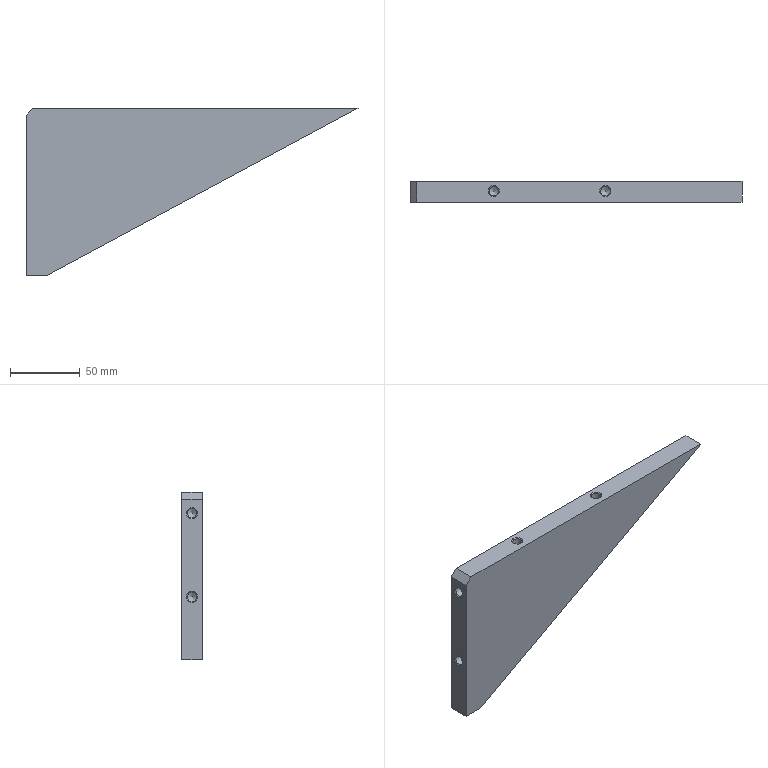Part | STEP file | YBQDJ-FLJ-6 | 1 solid | 19 faces | box 237.857 x 15 x 120 mm | volume 224363 mm3 | cone 8 | plane 7 | cylinder 4 | commonest cylinder face diameters 6.8 x4
STEP:
#1=CARTESIAN_POINT('',(0.,0.,0.));
#2=DIRECTION('',(0.,0.,1.));
#3=DIRECTION('',(1.,0.,0.));
#4=AXIS2_PLACEMENT_3D('',#1,#2,#3);
#5=CARTESIAN_POINT('',(486.5,-270.,-240.));
#6=VERTEX_POINT('',#5);
#7=CARTESIAN_POINT('',(486.5,-270.,-355.));
#8=VERTEX_POINT('',#7);
#9=CARTESIAN_POINT('',(486.5,-270.,-235.));
#10=DIRECTION('',(0.,0.,-1.));
#11=VECTOR('',#10,1.);
#12=LINE('',#9,#11);
#13=CARTESIAN_POINT('',(666.5,-270.,-395.));
#14=DIRECTION('',(0.,-1.,0.));
#15=DIRECTION('',(0.,0.,-1.));
#16=AXIS2_PLACEMENT_3D('',#13,#14,#15);
#17=PLANE('',#16);
#18=CARTESIAN_POINT('',(-160.,-180.));
#19=DIRECTION('',(1.,0.));
#20=VECTOR('',#19,1.);
#21=LINE('',#18,#20);
#22=(GEOMETRIC_REPRESENTATION_CONTEXT(2)PARAMETRIC_REPRESENTATION_CONTEXT()REPRESENTATION_CONTEXT('',''));
#23=DEFINITIONAL_REPRESENTATION('',(#21),#22);
#24=PCURVE('',#17,#23);
#25=CARTESIAN_POINT('',(486.5,-136.5,-235.));
#26=DIRECTION('',(-1.,0.,0.));
#27=DIRECTION('',(0.,0.,1.));
#28=AXIS2_PLACEMENT_3D('',#25,#26,#27);
#29=PLANE('',#28);
#30=CARTESIAN_POINT('',(0.,-133.5));
#31=DIRECTION('',(-1.,0.));
#32=VECTOR('',#31,1.);
#33=LINE('',#30,#32);
#34=(GEOMETRIC_REPRESENTATION_CONTEXT(2)PARAMETRIC_REPRESENTATION_CONTEXT()REPRESENTATION_CONTEXT('',''));
#35=DEFINITIONAL_REPRESENTATION('',(#33),#34);
#36=PCURVE('',#29,#35);
#37=SURFACE_CURVE('',#12,(#24,#36),.PCURVE_S1.);
#38=EDGE_CURVE('',#6,#8,#37,.T.);
#39=ORIENTED_EDGE('',*,*,#38,.F.);
#40=CARTESIAN_POINT('',(491.5,-270.,-235.));
#41=VERTEX_POINT('',#40);
#42=CARTESIAN_POINT('',(499.,-270.,-227.5));
#43=DIRECTION('',(0.7071,0.,0.7071));
#44=VECTOR('',#43,1.);
#45=LINE('',#42,#44);
#46=CARTESIAN_POINT('',(-167.5,-167.5));
#47=DIRECTION('',(-0.7071,0.7071));
#48=VECTOR('',#47,1.);
#49=LINE('',#46,#48);
#50=(GEOMETRIC_REPRESENTATION_CONTEXT(2)PARAMETRIC_REPRESENTATION_CONTEXT()REPRESENTATION_CONTEXT('',''));
#51=DEFINITIONAL_REPRESENTATION('',(#49),#50);
#52=PCURVE('',#17,#51);
#53=CARTESIAN_POINT('',(491.5,-136.5,-235.));
#54=DIRECTION('',(0.7071,0.,-0.7071));
#55=DIRECTION('',(0.,-1.,0.));
#56=AXIS2_PLACEMENT_3D('',#53,#54,#55);
#57=PLANE('',#56);
#58=CARTESIAN_POINT('',(133.5,-10.607));
#59=DIRECTION('',(0.,-1.));
#60=VECTOR('',#59,1.);
#61=LINE('',#58,#60);
#62=(GEOMETRIC_REPRESENTATION_CONTEXT(2)PARAMETRIC_REPRESENTATION_CONTEXT()REPRESENTATION_CONTEXT('',''));
#63=DEFINITIONAL_REPRESENTATION('',(#61),#62);
#64=PCURVE('',#57,#63);
#65=SURFACE_CURVE('',#45,(#52,#64),.PCURVE_S1.);
#66=EDGE_CURVE('',#6,#41,#65,.T.);
#67=ORIENTED_EDGE('',*,*,#66,.T.);
#68=CARTESIAN_POINT('',(724.357,-270.,-235.));
#69=VERTEX_POINT('',#68);
#70=CARTESIAN_POINT('',(696.5,-270.,-235.));
#71=DIRECTION('',(-1.,0.,0.));
#72=VECTOR('',#71,1.);
#73=LINE('',#70,#72);
#74=CARTESIAN_POINT('',(-160.,30.));
#75=DIRECTION('',(0.,-1.));
#76=VECTOR('',#75,1.);
#77=LINE('',#74,#76);
#78=(GEOMETRIC_REPRESENTATION_CONTEXT(2)PARAMETRIC_REPRESENTATION_CONTEXT()REPRESENTATION_CONTEXT('',''));
#79=DEFINITIONAL_REPRESENTATION('',(#77),#78);
#80=PCURVE('',#17,#79);
#81=CARTESIAN_POINT('',(696.5,-136.5,-235.));
#82=DIRECTION('',(0.,0.,1.));
#83=DIRECTION('',(1.,0.,0.));
#84=AXIS2_PLACEMENT_3D('',#81,#82,#83);
#85=PLANE('',#84);
#86=CARTESIAN_POINT('',(0.,-133.5));
#87=DIRECTION('',(-1.,0.));
#88=VECTOR('',#87,1.);
#89=LINE('',#86,#88);
#90=(GEOMETRIC_REPRESENTATION_CONTEXT(2)PARAMETRIC_REPRESENTATION_CONTEXT()REPRESENTATION_CONTEXT('',''));
#91=DEFINITIONAL_REPRESENTATION('',(#89),#90);
#92=PCURVE('',#85,#91);
#93=SURFACE_CURVE('',#73,(#80,#92),.PCURVE_S1.);
#94=EDGE_CURVE('',#69,#41,#93,.T.);
#95=ORIENTED_EDGE('',*,*,#94,.F.);
#96=CARTESIAN_POINT('',(501.5,-270.,-355.));
#97=VERTEX_POINT('',#96);
#98=CARTESIAN_POINT('',(501.5,-270.,-355.));
#99=DIRECTION('',(0.8805,0.,0.4741));
#100=VECTOR('',#99,1.);
#101=LINE('',#98,#100);
#102=CARTESIAN_POINT('',(-40.,-165.));
#103=DIRECTION('',(-0.4741,0.8805));
#104=VECTOR('',#103,1.);
#105=LINE('',#102,#104);
#106=(GEOMETRIC_REPRESENTATION_CONTEXT(2)PARAMETRIC_REPRESENTATION_CONTEXT()REPRESENTATION_CONTEXT('',''));
#107=DEFINITIONAL_REPRESENTATION('',(#105),#106);
#108=PCURVE('',#17,#107);
#109=CARTESIAN_POINT('',(501.5,-136.5,-355.));
#110=DIRECTION('',(0.4741,0.,-0.8805));
#111=DIRECTION('',(-0.8805,0.,-0.4741));
#112=AXIS2_PLACEMENT_3D('',#109,#110,#111);
#113=PLANE('',#112);
#114=CARTESIAN_POINT('',(0.,-133.5));
#115=DIRECTION('',(-1.,0.));
#116=VECTOR('',#115,1.);
#117=LINE('',#114,#116);
#118=(GEOMETRIC_REPRESENTATION_CONTEXT(2)PARAMETRIC_REPRESENTATION_CONTEXT()REPRESENTATION_CONTEXT('',''));
#119=DEFINITIONAL_REPRESENTATION('',(#117),#118);
#120=PCURVE('',#113,#119);
#121=SURFACE_CURVE('',#101,(#108,#120),.PCURVE_S1.);
#122=EDGE_CURVE('',#97,#69,#121,.T.);
#123=ORIENTED_EDGE('',*,*,#122,.F.);
#124=CARTESIAN_POINT('',(486.5,-270.,-355.));
#125=DIRECTION('',(1.,0.,0.));
#126=VECTOR('',#125,1.);
#127=LINE('',#124,#126);
#128=CARTESIAN_POINT('',(-40.,-180.));
#129=DIRECTION('',(0.,1.));
#130=VECTOR('',#129,1.);
#131=LINE('',#128,#130);
#132=(GEOMETRIC_REPRESENTATION_CONTEXT(2)PARAMETRIC_REPRESENTATION_CONTEXT()REPRESENTATION_CONTEXT('',''));
#133=DEFINITIONAL_REPRESENTATION('',(#131),#132);
#134=PCURVE('',#17,#133);
#135=CARTESIAN_POINT('',(486.5,-136.5,-355.));
#136=DIRECTION('',(0.,0.,-1.));
#137=DIRECTION('',(-1.,0.,0.));
#138=AXIS2_PLACEMENT_3D('',#135,#136,#137);
#139=PLANE('',#138);
#140=CARTESIAN_POINT('',(0.,-133.5));
#141=DIRECTION('',(-1.,0.));
#142=VECTOR('',#141,1.);
#143=LINE('',#140,#142);
#144=(GEOMETRIC_REPRESENTATION_CONTEXT(2)PARAMETRIC_REPRESENTATION_CONTEXT()REPRESENTATION_CONTEXT('',''));
#145=DEFINITIONAL_REPRESENTATION('',(#143),#144);
#146=PCURVE('',#139,#145);
#147=SURFACE_CURVE('',#127,(#134,#146),.PCURVE_S1.);
#148=EDGE_CURVE('',#8,#97,#147,.T.);
#149=ORIENTED_EDGE('',*,*,#148,.F.);
#150=EDGE_LOOP('',(#39,#67,#95,#123,#149));
#151=FACE_BOUND('',#150,.T.);
#152=ADVANCED_FACE('',(#151),#17,.F.);
#153=CARTESIAN_POINT('',(486.5,-285.,-355.));
#154=VERTEX_POINT('',#153);
#155=CARTESIAN_POINT('',(486.5,-136.5,-355.));
#156=DIRECTION('',(0.,-1.,0.));
#157=VECTOR('',#156,1.);
#158=LINE('',#155,#157);
#159=CARTESIAN_POINT('',(0.,0.));
#160=DIRECTION('',(0.,-1.));
#161=VECTOR('',#160,1.);
#162=LINE('',#159,#161);
#163=(GEOMETRIC_REPRESENTATION_CONTEXT(2)PARAMETRIC_REPRESENTATION_CONTEXT()REPRESENTATION_CONTEXT('',''));
#164=DEFINITIONAL_REPRESENTATION('',(#162),#163);
#165=PCURVE('',#139,#164);
#166=CARTESIAN_POINT('',(-120.,0.));
#167=DIRECTION('',(0.,-1.));
#168=VECTOR('',#167,1.);
#169=LINE('',#166,#168);
#170=(GEOMETRIC_REPRESENTATION_CONTEXT(2)PARAMETRIC_REPRESENTATION_CONTEXT()REPRESENTATION_CONTEXT('',''));
#171=DEFINITIONAL_REPRESENTATION('',(#169),#170);
#172=PCURVE('',#29,#171);
#173=SURFACE_CURVE('',#158,(#165,#172),.PCURVE_S1.);
#174=EDGE_CURVE('',#8,#154,#173,.T.);
#175=ORIENTED_EDGE('',*,*,#174,.F.);
#176=ORIENTED_EDGE('',*,*,#148,.T.);
#177=CARTESIAN_POINT('',(501.5,-285.,-355.));
#178=VERTEX_POINT('',#177);
#179=CARTESIAN_POINT('',(501.5,-136.5,-355.));
#180=DIRECTION('',(0.,-1.,0.));
#181=VECTOR('',#180,1.);
#182=LINE('',#179,#181);
#183=CARTESIAN_POINT('',(-15.,0.));
#184=DIRECTION('',(0.,-1.));
#185=VECTOR('',#184,1.);
#186=LINE('',#183,#185);
#187=(GEOMETRIC_REPRESENTATION_CONTEXT(2)PARAMETRIC_REPRESENTATION_CONTEXT()REPRESENTATION_CONTEXT('',''));
#188=DEFINITIONAL_REPRESENTATION('',(#186),#187);
#189=PCURVE('',#139,#188);
#190=CARTESIAN_POINT('',(0.,0.));
#191=DIRECTION('',(0.,-1.));
#192=VECTOR('',#191,1.);
#193=LINE('',#190,#192);
#194=(GEOMETRIC_REPRESENTATION_CONTEXT(2)PARAMETRIC_REPRESENTATION_CONTEXT()REPRESENTATION_CONTEXT('',''));
#195=DEFINITIONAL_REPRESENTATION('',(#193),#194);
#196=PCURVE('',#113,#195);
#197=SURFACE_CURVE('',#182,(#189,#196),.PCURVE_S1.);
#198=EDGE_CURVE('',#97,#178,#197,.T.);
#199=ORIENTED_EDGE('',*,*,#198,.T.);
#200=CARTESIAN_POINT('',(486.5,-285.,-355.));
#201=DIRECTION('',(1.,0.,0.));
#202=VECTOR('',#201,1.);
#203=LINE('',#200,#202);
#204=CARTESIAN_POINT('',(0.,-148.5));
#205=DIRECTION('',(-1.,0.));
#206=VECTOR('',#205,1.);
#207=LINE('',#204,#206);
#208=(GEOMETRIC_REPRESENTATION_CONTEXT(2)PARAMETRIC_REPRESENTATION_CONTEXT()REPRESENTATION_CONTEXT('',''));
#209=DEFINITIONAL_REPRESENTATION('',(#207),#208);
#210=PCURVE('',#139,#209);
#211=CARTESIAN_POINT('',(-13.5,-285.,-95.));
#212=DIRECTION('',(0.,1.,0.));
#213=DIRECTION('',(0.,0.,1.));
#214=AXIS2_PLACEMENT_3D('',#211,#212,#213);
#215=PLANE('',#214);
#216=CARTESIAN_POINT('',(-260.,500.));
#217=DIRECTION('',(0.,1.));
#218=VECTOR('',#217,1.);
#219=LINE('',#216,#218);
#220=(GEOMETRIC_REPRESENTATION_CONTEXT(2)PARAMETRIC_REPRESENTATION_CONTEXT()REPRESENTATION_CONTEXT('',''));
#221=DEFINITIONAL_REPRESENTATION('',(#219),#220);
#222=PCURVE('',#215,#221);
#223=SURFACE_CURVE('',#203,(#210,#222),.PCURVE_S1.);
#224=EDGE_CURVE('',#154,#178,#223,.T.);
#225=ORIENTED_EDGE('',*,*,#224,.F.);
#226=EDGE_LOOP('',(#175,#176,#199,#225));
#227=FACE_BOUND('',#226,.T.);
#228=ADVANCED_FACE('',(#227),#139,.T.);
#229=ORIENTED_EDGE('',*,*,#198,.F.);
#230=ORIENTED_EDGE('',*,*,#122,.T.);
#231=CARTESIAN_POINT('',(724.357,-285.,-235.));
#232=VERTEX_POINT('',#231);
#233=CARTESIAN_POINT('',(724.357,-136.5,-235.));
#234=DIRECTION('',(0.,1.,0.));
#235=VECTOR('',#234,1.);
#236=LINE('',#233,#235);
#237=CARTESIAN_POINT('',(-253.111,0.));
#238=DIRECTION('',(0.,1.));
#239=VECTOR('',#238,1.);
#240=LINE('',#237,#239);
#241=(GEOMETRIC_REPRESENTATION_CONTEXT(2)PARAMETRIC_REPRESENTATION_CONTEXT()REPRESENTATION_CONTEXT('',''));
#242=DEFINITIONAL_REPRESENTATION('',(#240),#241);
#243=PCURVE('',#113,#242);
#244=CARTESIAN_POINT('',(27.857,0.));
#245=DIRECTION('',(0.,1.));
#246=VECTOR('',#245,1.);
#247=LINE('',#244,#246);
#248=(GEOMETRIC_REPRESENTATION_CONTEXT(2)PARAMETRIC_REPRESENTATION_CONTEXT()REPRESENTATION_CONTEXT('',''));
#249=DEFINITIONAL_REPRESENTATION('',(#247),#248);
#250=PCURVE('',#85,#249);
#251=SURFACE_CURVE('',#236,(#243,#250),.PCURVE_S1.);
#252=EDGE_CURVE('',#232,#69,#251,.T.);
#253=ORIENTED_EDGE('',*,*,#252,.F.);
#254=CARTESIAN_POINT('',(501.5,-285.,-355.));
#255=DIRECTION('',(0.8805,0.,0.4741));
#256=VECTOR('',#255,1.);
#257=LINE('',#254,#256);
#258=CARTESIAN_POINT('',(0.,-148.5));
#259=DIRECTION('',(-1.,0.));
#260=VECTOR('',#259,1.);
#261=LINE('',#258,#260);
#262=(GEOMETRIC_REPRESENTATION_CONTEXT(2)PARAMETRIC_REPRESENTATION_CONTEXT()REPRESENTATION_CONTEXT('',''));
#263=DEFINITIONAL_REPRESENTATION('',(#261),#262);
#264=PCURVE('',#113,#263);
#265=CARTESIAN_POINT('',(-260.,515.));
#266=DIRECTION('',(0.4741,0.8805));
#267=VECTOR('',#266,1.);
#268=LINE('',#265,#267);
#269=(GEOMETRIC_REPRESENTATION_CONTEXT(2)PARAMETRIC_REPRESENTATION_CONTEXT()REPRESENTATION_CONTEXT('',''));
#270=DEFINITIONAL_REPRESENTATION('',(#268),#269);
#271=PCURVE('',#215,#270);
#272=SURFACE_CURVE('',#257,(#264,#271),.PCURVE_S1.);
#273=EDGE_CURVE('',#178,#232,#272,.T.);
#274=ORIENTED_EDGE('',*,*,#273,.F.);
#275=EDGE_LOOP('',(#229,#230,#253,#274));
#276=FACE_BOUND('',#275,.T.);
#277=ADVANCED_FACE('',(#276),#113,.T.);
#278=CARTESIAN_POINT('',(491.5,-285.,-235.));
#279=VERTEX_POINT('',#278);
#280=CARTESIAN_POINT('',(696.5,-285.,-235.));
#281=DIRECTION('',(-1.,0.,0.));
#282=VECTOR('',#281,1.);
#283=LINE('',#280,#282);
#284=CARTESIAN_POINT('',(-140.,710.));
#285=DIRECTION('',(0.,-1.));
#286=VECTOR('',#285,1.);
#287=LINE('',#284,#286);
#288=(GEOMETRIC_REPRESENTATION_CONTEXT(2)PARAMETRIC_REPRESENTATION_CONTEXT()REPRESENTATION_CONTEXT('',''));
#289=DEFINITIONAL_REPRESENTATION('',(#287),#288);
#290=PCURVE('',#215,#289);
#291=CARTESIAN_POINT('',(0.,-148.5));
#292=DIRECTION('',(-1.,0.));
#293=VECTOR('',#292,1.);
#294=LINE('',#291,#293);
#295=(GEOMETRIC_REPRESENTATION_CONTEXT(2)PARAMETRIC_REPRESENTATION_CONTEXT()REPRESENTATION_CONTEXT('',''));
#296=DEFINITIONAL_REPRESENTATION('',(#294),#295);
#297=PCURVE('',#85,#296);
#298=SURFACE_CURVE('',#283,(#290,#297),.PCURVE_S1.);
#299=EDGE_CURVE('',#232,#279,#298,.T.);
#300=ORIENTED_EDGE('',*,*,#299,.T.);
#301=CARTESIAN_POINT('',(486.5,-285.,-240.));
#302=VERTEX_POINT('',#301);
#303=CARTESIAN_POINT('',(491.5,-285.,-235.));
#304=DIRECTION('',(-0.7071,0.,-0.7071));
#305=VECTOR('',#304,1.);
#306=LINE('',#303,#305);
#307=CARTESIAN_POINT('',(-140.,505.));
#308=DIRECTION('',(-0.7071,-0.7071));
#309=VECTOR('',#308,1.);
#310=LINE('',#307,#309);
#311=(GEOMETRIC_REPRESENTATION_CONTEXT(2)PARAMETRIC_REPRESENTATION_CONTEXT()REPRESENTATION_CONTEXT('',''));
#312=DEFINITIONAL_REPRESENTATION('',(#310),#311);
#313=PCURVE('',#215,#312);
#314=CARTESIAN_POINT('',(148.5,0.));
#315=DIRECTION('',(0.,1.));
#316=VECTOR('',#315,1.);
#317=LINE('',#314,#316);
#318=(GEOMETRIC_REPRESENTATION_CONTEXT(2)PARAMETRIC_REPRESENTATION_CONTEXT()REPRESENTATION_CONTEXT('',''));
#319=DEFINITIONAL_REPRESENTATION('',(#317),#318);
#320=PCURVE('',#57,#319);
#321=SURFACE_CURVE('',#306,(#313,#320),.PCURVE_S1.);
#322=EDGE_CURVE('',#279,#302,#321,.T.);
#323=ORIENTED_EDGE('',*,*,#322,.T.);
#324=CARTESIAN_POINT('',(486.5,-285.,-235.));
#325=DIRECTION('',(0.,0.,-1.));
#326=VECTOR('',#325,1.);
#327=LINE('',#324,#326);
#328=CARTESIAN_POINT('',(-140.,500.));
#329=DIRECTION('',(-1.,0.));
#330=VECTOR('',#329,1.);
#331=LINE('',#328,#330);
#332=(GEOMETRIC_REPRESENTATION_CONTEXT(2)PARAMETRIC_REPRESENTATION_CONTEXT()REPRESENTATION_CONTEXT('',''));
#333=DEFINITIONAL_REPRESENTATION('',(#331),#332);
#334=PCURVE('',#215,#333);
#335=CARTESIAN_POINT('',(0.,-148.5));
#336=DIRECTION('',(-1.,0.));
#337=VECTOR('',#336,1.);
#338=LINE('',#335,#337);
#339=(GEOMETRIC_REPRESENTATION_CONTEXT(2)PARAMETRIC_REPRESENTATION_CONTEXT()REPRESENTATION_CONTEXT('',''));
#340=DEFINITIONAL_REPRESENTATION('',(#338),#339);
#341=PCURVE('',#29,#340);
#342=SURFACE_CURVE('',#327,(#334,#341),.PCURVE_S1.);
#343=EDGE_CURVE('',#302,#154,#342,.T.);
#344=ORIENTED_EDGE('',*,*,#343,.T.);
#345=ORIENTED_EDGE('',*,*,#224,.T.);
#346=ORIENTED_EDGE('',*,*,#273,.T.);
#347=EDGE_LOOP('',(#300,#323,#344,#345,#346));
#348=FACE_BOUND('',#347,.T.);
#349=ADVANCED_FACE('',(#348),#215,.F.);
#350=CARTESIAN_POINT('',(486.5,-277.5,-306.));
#351=VERTEX_POINT('',#350);
#352=CARTESIAN_POINT('',(486.5,-277.5,-310.));
#353=DIRECTION('',(1.,0.,0.));
#354=DIRECTION('',(0.,0.,1.));
#355=AXIS2_PLACEMENT_3D('',#352,#353,#354);
#356=CIRCLE('',#355,4.);
#357=CARTESIAN_POINT('',(-71.,-141.));
#358=CARTESIAN_POINT('',(-71.,-147.928));
#359=CARTESIAN_POINT('',(-77.,-144.464));
#360=CARTESIAN_POINT('',(-83.,-141.));
#361=CARTESIAN_POINT('',(-77.,-137.536));
#362=CARTESIAN_POINT('',(-71.,-134.072));
#363=CARTESIAN_POINT('',(-71.,-141.));
#364=(BOUNDED_CURVE()B_SPLINE_CURVE(2,(#357,#358,#359,#360,#361,#362,#363),.UNSPECIFIED.,.T.,.F.)B_SPLINE_CURVE_WITH_KNOTS((1,2,2,2,2,1),(-2.094,0.,2.094,4.189,6.283,8.378),.UNSPECIFIED.)CURVE()GEOMETRIC_REPRESENTATION_ITEM()RATIONAL_B_SPLINE_CURVE((1.,0.5,1.,0.5,1.,0.5,1.))REPRESENTATION_ITEM(''));
#365=(GEOMETRIC_REPRESENTATION_CONTEXT(2)PARAMETRIC_REPRESENTATION_CONTEXT()REPRESENTATION_CONTEXT('',''));
#366=DEFINITIONAL_REPRESENTATION('',(#364),#365);
#367=PCURVE('',#29,#366);
#368=CARTESIAN_POINT('',(486.5,-277.5,-310.));
#369=DIRECTION('',(-1.,0.,0.));
#370=DIRECTION('',(0.,0.,1.));
#371=AXIS2_PLACEMENT_3D('',#368,#369,#370);
#372=CONICAL_SURFACE('',#371,4.,0.7854);
#373=CARTESIAN_POINT('',(6.283,0.));
#374=DIRECTION('',(-1.,0.));
#375=VECTOR('',#374,1.);
#376=LINE('',#373,#375);
#377=(GEOMETRIC_REPRESENTATION_CONTEXT(2)PARAMETRIC_REPRESENTATION_CONTEXT()REPRESENTATION_CONTEXT('',''));
#378=DEFINITIONAL_REPRESENTATION('',(#376),#377);
#379=PCURVE('',#372,#378);
#380=SURFACE_CURVE('',#356,(#367,#379),.PCURVE_S1.);
#381=EDGE_CURVE('',#351,#351,#380,.T.);
#382=ORIENTED_EDGE('',*,*,#381,.T.);
#383=EDGE_LOOP('',(#382));
#384=FACE_BOUND('',#383,.T.);
#385=CARTESIAN_POINT('',(486.5,-277.5,-246.));
#386=VERTEX_POINT('',#385);
#387=CARTESIAN_POINT('',(486.5,-277.5,-250.));
#388=DIRECTION('',(1.,0.,0.));
#389=DIRECTION('',(0.,0.,1.));
#390=AXIS2_PLACEMENT_3D('',#387,#388,#389);
#391=CIRCLE('',#390,4.);
#392=CARTESIAN_POINT('',(-11.,-141.));
#393=CARTESIAN_POINT('',(-11.,-147.928));
#394=CARTESIAN_POINT('',(-17.,-144.464));
#395=CARTESIAN_POINT('',(-23.,-141.));
#396=CARTESIAN_POINT('',(-17.,-137.536));
#397=CARTESIAN_POINT('',(-11.,-134.072));
#398=CARTESIAN_POINT('',(-11.,-141.));
#399=(BOUNDED_CURVE()B_SPLINE_CURVE(2,(#392,#393,#394,#395,#396,#397,#398),.UNSPECIFIED.,.T.,.F.)B_SPLINE_CURVE_WITH_KNOTS((1,2,2,2,2,1),(-2.094,0.,2.094,4.189,6.283,8.378),.UNSPECIFIED.)CURVE()GEOMETRIC_REPRESENTATION_ITEM()RATIONAL_B_SPLINE_CURVE((1.,0.5,1.,0.5,1.,0.5,1.))REPRESENTATION_ITEM(''));
#400=(GEOMETRIC_REPRESENTATION_CONTEXT(2)PARAMETRIC_REPRESENTATION_CONTEXT()REPRESENTATION_CONTEXT('',''));
#401=DEFINITIONAL_REPRESENTATION('',(#399),#400);
#402=PCURVE('',#29,#401);
#403=CARTESIAN_POINT('',(486.5,-277.5,-250.));
#404=DIRECTION('',(-1.,0.,0.));
#405=DIRECTION('',(0.,0.,1.));
#406=AXIS2_PLACEMENT_3D('',#403,#404,#405);
#407=CONICAL_SURFACE('',#406,4.,0.7854);
#408=CARTESIAN_POINT('',(6.283,0.));
#409=DIRECTION('',(-1.,0.));
#410=VECTOR('',#409,1.);
#411=LINE('',#408,#410);
#412=(GEOMETRIC_REPRESENTATION_CONTEXT(2)PARAMETRIC_REPRESENTATION_CONTEXT()REPRESENTATION_CONTEXT('',''));
#413=DEFINITIONAL_REPRESENTATION('',(#411),#412);
#414=PCURVE('',#407,#413);
#415=SURFACE_CURVE('',#391,(#402,#414),.PCURVE_S1.);
#416=EDGE_CURVE('',#386,#386,#415,.T.);
#417=ORIENTED_EDGE('',*,*,#416,.T.);
#418=EDGE_LOOP('',(#417));
#419=FACE_BOUND('',#418,.T.);
#420=ORIENTED_EDGE('',*,*,#343,.F.);
#421=CARTESIAN_POINT('',(486.5,-136.5,-240.));
#422=DIRECTION('',(0.,1.,0.));
#423=VECTOR('',#422,1.);
#424=LINE('',#421,#423);
#425=CARTESIAN_POINT('',(-5.,0.));
#426=DIRECTION('',(0.,1.));
#427=VECTOR('',#426,1.);
#428=LINE('',#425,#427);
#429=(GEOMETRIC_REPRESENTATION_CONTEXT(2)PARAMETRIC_REPRESENTATION_CONTEXT()REPRESENTATION_CONTEXT('',''));
#430=DEFINITIONAL_REPRESENTATION('',(#428),#429);
#431=PCURVE('',#29,#430);
#432=CARTESIAN_POINT('',(0.,7.071));
#433=DIRECTION('',(-1.,0.));
#434=VECTOR('',#433,1.);
#435=LINE('',#432,#434);
#436=(GEOMETRIC_REPRESENTATION_CONTEXT(2)PARAMETRIC_REPRESENTATION_CONTEXT()REPRESENTATION_CONTEXT('',''));
#437=DEFINITIONAL_REPRESENTATION('',(#435),#436);
#438=PCURVE('',#57,#437);
#439=SURFACE_CURVE('',#424,(#431,#438),.PCURVE_S1.);
#440=EDGE_CURVE('',#302,#6,#439,.T.);
#441=ORIENTED_EDGE('',*,*,#440,.T.);
#442=ORIENTED_EDGE('',*,*,#38,.T.);
#443=ORIENTED_EDGE('',*,*,#174,.T.);
#444=EDGE_LOOP('',(#420,#441,#442,#443));
#445=FACE_BOUND('',#444,.T.);
#446=ADVANCED_FACE('',(#384,#419,#445),#29,.T.);
#447=CARTESIAN_POINT('',(630.5,-277.01,-235.));
#448=VERTEX_POINT('',#447);
#449=CARTESIAN_POINT('',(626.5,-277.01,-235.));
#450=DIRECTION('',(0.,0.,-1.));
#451=DIRECTION('',(1.,0.,0.));
#452=AXIS2_PLACEMENT_3D('',#449,#450,#451);
#453=CIRCLE('',#452,4.);
#454=CARTESIAN_POINT('',(-66.,-140.51));
#455=CARTESIAN_POINT('',(-66.,-147.439));
#456=CARTESIAN_POINT('',(-72.,-143.974));
#457=CARTESIAN_POINT('',(-78.,-140.51));
#458=CARTESIAN_POINT('',(-72.,-137.046));
#459=CARTESIAN_POINT('',(-66.,-133.582));
#460=CARTESIAN_POINT('',(-66.,-140.51));
#461=(BOUNDED_CURVE()B_SPLINE_CURVE(2,(#454,#455,#456,#457,#458,#459,#460),.UNSPECIFIED.,.T.,.F.)B_SPLINE_CURVE_WITH_KNOTS((1,2,2,2,2,1),(-2.094,0.,2.094,4.189,6.283,8.378),.UNSPECIFIED.)CURVE()GEOMETRIC_REPRESENTATION_ITEM()RATIONAL_B_SPLINE_CURVE((1.,0.5,1.,0.5,1.,0.5,1.))REPRESENTATION_ITEM(''));
#462=(GEOMETRIC_REPRESENTATION_CONTEXT(2)PARAMETRIC_REPRESENTATION_CONTEXT()REPRESENTATION_CONTEXT('',''));
#463=DEFINITIONAL_REPRESENTATION('',(#461),#462);
#464=PCURVE('',#85,#463);
#465=CARTESIAN_POINT('',(626.5,-277.01,-235.));
#466=DIRECTION('',(0.,0.,1.));
#467=DIRECTION('',(1.,0.,0.));
#468=AXIS2_PLACEMENT_3D('',#465,#466,#467);
#469=CONICAL_SURFACE('',#468,4.,0.7854);
#470=CARTESIAN_POINT('',(6.283,0.));
#471=DIRECTION('',(-1.,0.));
#472=VECTOR('',#471,1.);
#473=LINE('',#470,#472);
#474=(GEOMETRIC_REPRESENTATION_CONTEXT(2)PARAMETRIC_REPRESENTATION_CONTEXT()REPRESENTATION_CONTEXT('',''));
#475=DEFINITIONAL_REPRESENTATION('',(#473),#474);
#476=PCURVE('',#469,#475);
#477=SURFACE_CURVE('',#453,(#464,#476),.PCURVE_S1.);
#478=EDGE_CURVE('',#448,#448,#477,.T.);
#479=ORIENTED_EDGE('',*,*,#478,.T.);
#480=EDGE_LOOP('',(#479));
#481=FACE_BOUND('',#480,.T.);
#482=CARTESIAN_POINT('',(550.5,-277.01,-235.));
#483=VERTEX_POINT('',#482);
#484=CARTESIAN_POINT('',(546.5,-277.01,-235.));
#485=DIRECTION('',(0.,0.,-1.));
#486=DIRECTION('',(1.,0.,0.));
#487=AXIS2_PLACEMENT_3D('',#484,#485,#486);
#488=CIRCLE('',#487,4.);
#489=CARTESIAN_POINT('',(-146.,-140.51));
#490=CARTESIAN_POINT('',(-146.,-147.439));
#491=CARTESIAN_POINT('',(-152.,-143.974));
#492=CARTESIAN_POINT('',(-158.,-140.51));
#493=CARTESIAN_POINT('',(-152.,-137.046));
#494=CARTESIAN_POINT('',(-146.,-133.582));
#495=CARTESIAN_POINT('',(-146.,-140.51));
#496=(BOUNDED_CURVE()B_SPLINE_CURVE(2,(#489,#490,#491,#492,#493,#494,#495),.UNSPECIFIED.,.T.,.F.)B_SPLINE_CURVE_WITH_KNOTS((1,2,2,2,2,1),(-2.094,0.,2.094,4.189,6.283,8.378),.UNSPECIFIED.)CURVE()GEOMETRIC_REPRESENTATION_ITEM()RATIONAL_B_SPLINE_CURVE((1.,0.5,1.,0.5,1.,0.5,1.))REPRESENTATION_ITEM(''));
#497=(GEOMETRIC_REPRESENTATION_CONTEXT(2)PARAMETRIC_REPRESENTATION_CONTEXT()REPRESENTATION_CONTEXT('',''));
#498=DEFINITIONAL_REPRESENTATION('',(#496),#497);
#499=PCURVE('',#85,#498);
#500=CARTESIAN_POINT('',(546.5,-277.01,-235.));
#501=DIRECTION('',(0.,0.,1.));
#502=DIRECTION('',(1.,0.,0.));
#503=AXIS2_PLACEMENT_3D('',#500,#501,#502);
#504=CONICAL_SURFACE('',#503,4.,0.7854);
#505=CARTESIAN_POINT('',(6.283,0.));
#506=DIRECTION('',(-1.,0.));
#507=VECTOR('',#506,1.);
#508=LINE('',#505,#507);
#509=(GEOMETRIC_REPRESENTATION_CONTEXT(2)PARAMETRIC_REPRESENTATION_CONTEXT()REPRESENTATION_CONTEXT('',''));
#510=DEFINITIONAL_REPRESENTATION('',(#508),#509);
#511=PCURVE('',#504,#510);
#512=SURFACE_CURVE('',#488,(#499,#511),.PCURVE_S1.);
#513=EDGE_CURVE('',#483,#483,#512,.T.);
#514=ORIENTED_EDGE('',*,*,#513,.T.);
#515=EDGE_LOOP('',(#514));
#516=FACE_BOUND('',#515,.T.);
#517=ORIENTED_EDGE('',*,*,#94,.T.);
#518=CARTESIAN_POINT('',(491.5,-136.5,-235.));
#519=DIRECTION('',(0.,-1.,0.));
#520=VECTOR('',#519,1.);
#521=LINE('',#518,#520);
#522=CARTESIAN_POINT('',(-205.,0.));
#523=DIRECTION('',(0.,-1.));
#524=VECTOR('',#523,1.);
#525=LINE('',#522,#524);
#526=(GEOMETRIC_REPRESENTATION_CONTEXT(2)PARAMETRIC_REPRESENTATION_CONTEXT()REPRESENTATION_CONTEXT('',''));
#527=DEFINITIONAL_REPRESENTATION('',(#525),#526);
#528=PCURVE('',#85,#527);
#529=CARTESIAN_POINT('',(0.,0.));
#530=DIRECTION('',(1.,0.));
#531=VECTOR('',#530,1.);
#532=LINE('',#529,#531);
#533=(GEOMETRIC_REPRESENTATION_CONTEXT(2)PARAMETRIC_REPRESENTATION_CONTEXT()REPRESENTATION_CONTEXT('',''));
#534=DEFINITIONAL_REPRESENTATION('',(#532),#533);
#535=PCURVE('',#57,#534);
#536=SURFACE_CURVE('',#521,(#528,#535),.PCURVE_S1.);
#537=EDGE_CURVE('',#41,#279,#536,.T.);
#538=ORIENTED_EDGE('',*,*,#537,.T.);
#539=ORIENTED_EDGE('',*,*,#299,.F.);
#540=ORIENTED_EDGE('',*,*,#252,.T.);
#541=EDGE_LOOP('',(#517,#538,#539,#540));
#542=FACE_BOUND('',#541,.T.);
#543=ADVANCED_FACE('',(#481,#516,#542),#85,.T.);
#544=CARTESIAN_POINT('',(549.9,-277.01,-255.));
#545=VERTEX_POINT('',#544);
#546=CARTESIAN_POINT('',(543.1,-277.01,-255.));
#547=VERTEX_POINT('',#546);
#548=CARTESIAN_POINT('',(546.5,-277.01,-255.));
#549=DIRECTION('',(0.,0.,1.));
#550=DIRECTION('',(-1.,0.,0.));
#551=AXIS2_PLACEMENT_3D('',#548,#549,#550);
#552=CIRCLE('',#551,3.4);
#553=CARTESIAN_POINT('',(546.5,-277.01,-255.));
#554=DIRECTION('',(0.,0.,1.));
#555=DIRECTION('',(1.,0.,0.));
#556=AXIS2_PLACEMENT_3D('',#553,#554,#555);
#557=CONICAL_SURFACE('',#556,3.4,1.03);
#558=CARTESIAN_POINT('',(-3.142,0.));
#559=DIRECTION('',(1.,0.));
#560=VECTOR('',#559,1.);
#561=LINE('',#558,#560);
#562=(GEOMETRIC_REPRESENTATION_CONTEXT(2)PARAMETRIC_REPRESENTATION_CONTEXT()REPRESENTATION_CONTEXT('',''));
#563=DEFINITIONAL_REPRESENTATION('',(#561),#562);
#564=PCURVE('',#557,#563);
#565=CARTESIAN_POINT('',(546.5,-277.01,-235.));
#566=DIRECTION('',(0.,0.,-1.));
#567=DIRECTION('',(-1.,0.,0.));
#568=AXIS2_PLACEMENT_3D('',#565,#566,#567);
#569=CYLINDRICAL_SURFACE('',#568,3.4);
#570=CARTESIAN_POINT('',(12.566,20.));
#571=DIRECTION('',(-1.,0.));
#572=VECTOR('',#571,1.);
#573=LINE('',#570,#572);
#574=(GEOMETRIC_REPRESENTATION_CONTEXT(2)PARAMETRIC_REPRESENTATION_CONTEXT()REPRESENTATION_CONTEXT('',''));
#575=DEFINITIONAL_REPRESENTATION('',(#573),#574);
#576=PCURVE('',#569,#575);
#577=SURFACE_CURVE('',#552,(#564,#576),.PCURVE_S1.);
#578=EDGE_CURVE('',#545,#547,#577,.T.);
#579=ORIENTED_EDGE('',*,*,#578,.F.);
#580=CARTESIAN_POINT('',(546.5,-277.01,-257.043));
#581=VERTEX_POINT('',#580);
#582=CARTESIAN_POINT('',(546.5,-277.01,-257.043));
#583=CARTESIAN_POINT('',(549.9,-277.01,-255.));
#584=B_SPLINE_CURVE_WITH_KNOTS('',1,(#582,#583),.UNSPECIFIED.,.F.,.F.,(2,2),(-3.967,0.),.PIECEWISE_BEZIER_KNOTS.);
#585=CARTESIAN_POINT('',(0.,0.));
#586=DIRECTION('',(0.,1.));
#587=VECTOR('',#586,1.);
#588=LINE('',#585,#587);
#589=(GEOMETRIC_REPRESENTATION_CONTEXT(2)PARAMETRIC_REPRESENTATION_CONTEXT()REPRESENTATION_CONTEXT('',''));
#590=DEFINITIONAL_REPRESENTATION('',(#588),#589);
#591=PCURVE('',#557,#590);
#592=CARTESIAN_POINT('',(6.283,0.));
#593=DIRECTION('',(0.,1.));
#594=VECTOR('',#593,1.);
#595=LINE('',#592,#594);
#596=(GEOMETRIC_REPRESENTATION_CONTEXT(2)PARAMETRIC_REPRESENTATION_CONTEXT()REPRESENTATION_CONTEXT('',''));
#597=DEFINITIONAL_REPRESENTATION('',(#595),#596);
#598=PCURVE('',#557,#597);
#599=SEAM_CURVE('',#584,(#591,#598),.PCURVE_S1.);
#600=EDGE_CURVE('',#581,#545,#599,.T.);
#601=ORIENTED_EDGE('',*,*,#600,.F.);
#602=ORIENTED_EDGE('',*,*,#600,.T.);
#603=CARTESIAN_POINT('',(546.5,-277.01,-255.));
#604=DIRECTION('',(0.,0.,1.));
#605=DIRECTION('',(-1.,0.,0.));
#606=AXIS2_PLACEMENT_3D('',#603,#604,#605);
#607=CIRCLE('',#606,3.4);
#608=CARTESIAN_POINT('',(3.142,0.));
#609=DIRECTION('',(1.,0.));
#610=VECTOR('',#609,1.);
#611=LINE('',#608,#610);
#612=(GEOMETRIC_REPRESENTATION_CONTEXT(2)PARAMETRIC_REPRESENTATION_CONTEXT()REPRESENTATION_CONTEXT('',''));
#613=DEFINITIONAL_REPRESENTATION('',(#611),#612);
#614=PCURVE('',#557,#613);
#615=CARTESIAN_POINT('',(6.283,20.));
#616=DIRECTION('',(-1.,0.));
#617=VECTOR('',#616,1.);
#618=LINE('',#615,#617);
#619=(GEOMETRIC_REPRESENTATION_CONTEXT(2)PARAMETRIC_REPRESENTATION_CONTEXT()REPRESENTATION_CONTEXT('',''));
#620=DEFINITIONAL_REPRESENTATION('',(#618),#619);
#621=PCURVE('',#569,#620);
#622=SURFACE_CURVE('',#607,(#614,#621),.PCURVE_S1.);
#623=EDGE_CURVE('',#547,#545,#622,.T.);
#624=ORIENTED_EDGE('',*,*,#623,.F.);
#625=EDGE_LOOP('',(#579,#601,#602,#624));
#626=FACE_BOUND('',#625,.F.);
#627=ADVANCED_FACE('',(#626),#557,.F.);
#628=CARTESIAN_POINT('',(549.9,-277.01,-235.6));
#629=VERTEX_POINT('',#628);
#630=CARTESIAN_POINT('',(546.5,-277.01,-235.6));
#631=DIRECTION('',(0.,0.,1.));
#632=DIRECTION('',(1.,0.,0.));
#633=AXIS2_PLACEMENT_3D('',#630,#631,#632);
#634=CIRCLE('',#633,3.4);
#635=CARTESIAN_POINT('',(9.425,0.6));
#636=DIRECTION('',(-1.,0.));
#637=VECTOR('',#636,1.);
#638=LINE('',#635,#637);
#639=(GEOMETRIC_REPRESENTATION_CONTEXT(2)PARAMETRIC_REPRESENTATION_CONTEXT()REPRESENTATION_CONTEXT('',''));
#640=DEFINITIONAL_REPRESENTATION('',(#638),#639);
#641=PCURVE('',#569,#640);
#642=CARTESIAN_POINT('',(0.,-0.6));
#643=DIRECTION('',(1.,0.));
#644=VECTOR('',#643,1.);
#645=LINE('',#642,#644);
#646=(GEOMETRIC_REPRESENTATION_CONTEXT(2)PARAMETRIC_REPRESENTATION_CONTEXT()REPRESENTATION_CONTEXT('',''));
#647=DEFINITIONAL_REPRESENTATION('',(#645),#646);
#648=PCURVE('',#504,#647);
#649=SURFACE_CURVE('',#634,(#641,#648),.PCURVE_S1.);
#650=EDGE_CURVE('',#629,#629,#649,.T.);
#651=ORIENTED_EDGE('',*,*,#650,.F.);
#652=CARTESIAN_POINT('',(549.9,-277.01,-235.6));
#653=CARTESIAN_POINT('',(549.9,-277.01,-255.));
#654=B_SPLINE_CURVE_WITH_KNOTS('',1,(#652,#653),.UNSPECIFIED.,.F.,.F.,(2,2),(0.6,20.),.PIECEWISE_BEZIER_KNOTS.);
#655=CARTESIAN_POINT('',(9.425,0.));
#656=DIRECTION('',(0.,1.));
#657=VECTOR('',#656,1.);
#658=LINE('',#655,#657);
#659=(GEOMETRIC_REPRESENTATION_CONTEXT(2)PARAMETRIC_REPRESENTATION_CONTEXT()REPRESENTATION_CONTEXT('',''));
#660=DEFINITIONAL_REPRESENTATION('',(#658),#659);
#661=PCURVE('',#569,#660);
#662=CARTESIAN_POINT('',(3.142,0.));
#663=DIRECTION('',(0.,1.));
#664=VECTOR('',#663,1.);
#665=LINE('',#662,#664);
#666=(GEOMETRIC_REPRESENTATION_CONTEXT(2)PARAMETRIC_REPRESENTATION_CONTEXT()REPRESENTATION_CONTEXT('',''));
#667=DEFINITIONAL_REPRESENTATION('',(#665),#666);
#668=PCURVE('',#569,#667);
#669=SEAM_CURVE('',#654,(#661,#668),.PCURVE_S1.);
#670=EDGE_CURVE('',#629,#545,#669,.T.);
#671=ORIENTED_EDGE('',*,*,#670,.T.);
#672=ORIENTED_EDGE('',*,*,#578,.T.);
#673=ORIENTED_EDGE('',*,*,#623,.T.);
#674=ORIENTED_EDGE('',*,*,#670,.F.);
#675=EDGE_LOOP('',(#651,#671,#672,#673,#674));
#676=FACE_BOUND('',#675,.F.);
#677=ADVANCED_FACE('',(#676),#569,.F.);
#678=ORIENTED_EDGE('',*,*,#650,.T.);
#679=CARTESIAN_POINT('',(549.9,-277.01,-235.6));
#680=CARTESIAN_POINT('',(550.5,-277.01,-235.));
#681=B_SPLINE_CURVE_WITH_KNOTS('',1,(#679,#680),.UNSPECIFIED.,.F.,.F.,(2,2),(-0.8485,0.),.PIECEWISE_BEZIER_KNOTS.);
#682=CARTESIAN_POINT('',(6.283,0.));
#683=DIRECTION('',(0.,1.));
#684=VECTOR('',#683,1.);
#685=LINE('',#682,#684);
#686=(GEOMETRIC_REPRESENTATION_CONTEXT(2)PARAMETRIC_REPRESENTATION_CONTEXT()REPRESENTATION_CONTEXT('',''));
#687=DEFINITIONAL_REPRESENTATION('',(#685),#686);
#688=PCURVE('',#504,#687);
#689=CARTESIAN_POINT('',(0.,0.));
#690=DIRECTION('',(0.,1.));
#691=VECTOR('',#690,1.);
#692=LINE('',#689,#691);
#693=(GEOMETRIC_REPRESENTATION_CONTEXT(2)PARAMETRIC_REPRESENTATION_CONTEXT()REPRESENTATION_CONTEXT('',''));
#694=DEFINITIONAL_REPRESENTATION('',(#692),#693);
#695=PCURVE('',#504,#694);
#696=SEAM_CURVE('',#681,(#688,#695),.PCURVE_S1.);
#697=EDGE_CURVE('',#629,#483,#696,.T.);
#698=ORIENTED_EDGE('',*,*,#697,.T.);
#699=ORIENTED_EDGE('',*,*,#513,.T.);
#700=ORIENTED_EDGE('',*,*,#697,.F.);
#701=EDGE_LOOP('',(#678,#698,#699,#700));
#702=FACE_BOUND('',#701,.F.);
#703=ADVANCED_FACE('',(#702),#504,.F.);
#704=CARTESIAN_POINT('',(629.9,-277.01,-255.));
#705=VERTEX_POINT('',#704);
#706=CARTESIAN_POINT('',(623.1,-277.01,-255.));
#707=VERTEX_POINT('',#706);
#708=CARTESIAN_POINT('',(626.5,-277.01,-255.));
#709=DIRECTION('',(0.,0.,1.));
#710=DIRECTION('',(-1.,0.,0.));
#711=AXIS2_PLACEMENT_3D('',#708,#709,#710);
#712=CIRCLE('',#711,3.4);
#713=CARTESIAN_POINT('',(626.5,-277.01,-255.));
#714=DIRECTION('',(0.,0.,1.));
#715=DIRECTION('',(1.,0.,0.));
#716=AXIS2_PLACEMENT_3D('',#713,#714,#715);
#717=CONICAL_SURFACE('',#716,3.4,1.03);
#718=CARTESIAN_POINT('',(-3.142,0.));
#719=DIRECTION('',(1.,0.));
#720=VECTOR('',#719,1.);
#721=LINE('',#718,#720);
#722=(GEOMETRIC_REPRESENTATION_CONTEXT(2)PARAMETRIC_REPRESENTATION_CONTEXT()REPRESENTATION_CONTEXT('',''));
#723=DEFINITIONAL_REPRESENTATION('',(#721),#722);
#724=PCURVE('',#717,#723);
#725=CARTESIAN_POINT('',(626.5,-277.01,-235.));
#726=DIRECTION('',(0.,0.,-1.));
#727=DIRECTION('',(-1.,0.,0.));
#728=AXIS2_PLACEMENT_3D('',#725,#726,#727);
#729=CYLINDRICAL_SURFACE('',#728,3.4);
#730=CARTESIAN_POINT('',(12.566,20.));
#731=DIRECTION('',(-1.,0.));
#732=VECTOR('',#731,1.);
#733=LINE('',#730,#732);
#734=(GEOMETRIC_REPRESENTATION_CONTEXT(2)PARAMETRIC_REPRESENTATION_CONTEXT()REPRESENTATION_CONTEXT('',''));
#735=DEFINITIONAL_REPRESENTATION('',(#733),#734);
#736=PCURVE('',#729,#735);
#737=SURFACE_CURVE('',#712,(#724,#736),.PCURVE_S1.);
#738=EDGE_CURVE('',#705,#707,#737,.T.);
#739=ORIENTED_EDGE('',*,*,#738,.F.);
#740=CARTESIAN_POINT('',(626.5,-277.01,-257.043));
#741=VERTEX_POINT('',#740);
#742=CARTESIAN_POINT('',(626.5,-277.01,-257.043));
#743=CARTESIAN_POINT('',(629.9,-277.01,-255.));
#744=B_SPLINE_CURVE_WITH_KNOTS('',1,(#742,#743),.UNSPECIFIED.,.F.,.F.,(2,2),(-3.967,0.),.PIECEWISE_BEZIER_KNOTS.);
#745=CARTESIAN_POINT('',(0.,0.));
#746=DIRECTION('',(0.,1.));
#747=VECTOR('',#746,1.);
#748=LINE('',#745,#747);
#749=(GEOMETRIC_REPRESENTATION_CONTEXT(2)PARAMETRIC_REPRESENTATION_CONTEXT()REPRESENTATION_CONTEXT('',''));
#750=DEFINITIONAL_REPRESENTATION('',(#748),#749);
#751=PCURVE('',#717,#750);
#752=CARTESIAN_POINT('',(6.283,0.));
#753=DIRECTION('',(0.,1.));
#754=VECTOR('',#753,1.);
#755=LINE('',#752,#754);
#756=(GEOMETRIC_REPRESENTATION_CONTEXT(2)PARAMETRIC_REPRESENTATION_CONTEXT()REPRESENTATION_CONTEXT('',''));
#757=DEFINITIONAL_REPRESENTATION('',(#755),#756);
#758=PCURVE('',#717,#757);
#759=SEAM_CURVE('',#744,(#751,#758),.PCURVE_S1.);
#760=EDGE_CURVE('',#741,#705,#759,.T.);
#761=ORIENTED_EDGE('',*,*,#760,.F.);
#762=ORIENTED_EDGE('',*,*,#760,.T.);
#763=CARTESIAN_POINT('',(626.5,-277.01,-255.));
#764=DIRECTION('',(0.,0.,1.));
#765=DIRECTION('',(-1.,0.,0.));
#766=AXIS2_PLACEMENT_3D('',#763,#764,#765);
#767=CIRCLE('',#766,3.4);
#768=CARTESIAN_POINT('',(3.142,0.));
#769=DIRECTION('',(1.,0.));
#770=VECTOR('',#769,1.);
#771=LINE('',#768,#770);
#772=(GEOMETRIC_REPRESENTATION_CONTEXT(2)PARAMETRIC_REPRESENTATION_CONTEXT()REPRESENTATION_CONTEXT('',''));
#773=DEFINITIONAL_REPRESENTATION('',(#771),#772);
#774=PCURVE('',#717,#773);
#775=CARTESIAN_POINT('',(6.283,20.));
#776=DIRECTION('',(-1.,0.));
#777=VECTOR('',#776,1.);
#778=LINE('',#775,#777);
#779=(GEOMETRIC_REPRESENTATION_CONTEXT(2)PARAMETRIC_REPRESENTATION_CONTEXT()REPRESENTATION_CONTEXT('',''));
#780=DEFINITIONAL_REPRESENTATION('',(#778),#779);
#781=PCURVE('',#729,#780);
#782=SURFACE_CURVE('',#767,(#774,#781),.PCURVE_S1.);
#783=EDGE_CURVE('',#707,#705,#782,.T.);
#784=ORIENTED_EDGE('',*,*,#783,.F.);
#785=EDGE_LOOP('',(#739,#761,#762,#784));
#786=FACE_BOUND('',#785,.F.);
#787=ADVANCED_FACE('',(#786),#717,.F.);
#788=CARTESIAN_POINT('',(629.9,-277.01,-235.6));
#789=VERTEX_POINT('',#788);
#790=CARTESIAN_POINT('',(626.5,-277.01,-235.6));
#791=DIRECTION('',(0.,0.,1.));
#792=DIRECTION('',(1.,0.,0.));
#793=AXIS2_PLACEMENT_3D('',#790,#791,#792);
#794=CIRCLE('',#793,3.4);
#795=CARTESIAN_POINT('',(9.425,0.6));
#796=DIRECTION('',(-1.,0.));
#797=VECTOR('',#796,1.);
#798=LINE('',#795,#797);
#799=(GEOMETRIC_REPRESENTATION_CONTEXT(2)PARAMETRIC_REPRESENTATION_CONTEXT()REPRESENTATION_CONTEXT('',''));
#800=DEFINITIONAL_REPRESENTATION('',(#798),#799);
#801=PCURVE('',#729,#800);
#802=CARTESIAN_POINT('',(0.,-0.6));
#803=DIRECTION('',(1.,0.));
#804=VECTOR('',#803,1.);
#805=LINE('',#802,#804);
#806=(GEOMETRIC_REPRESENTATION_CONTEXT(2)PARAMETRIC_REPRESENTATION_CONTEXT()REPRESENTATION_CONTEXT('',''));
#807=DEFINITIONAL_REPRESENTATION('',(#805),#806);
#808=PCURVE('',#469,#807);
#809=SURFACE_CURVE('',#794,(#801,#808),.PCURVE_S1.);
#810=EDGE_CURVE('',#789,#789,#809,.T.);
#811=ORIENTED_EDGE('',*,*,#810,.F.);
#812=CARTESIAN_POINT('',(629.9,-277.01,-235.6));
#813=CARTESIAN_POINT('',(629.9,-277.01,-255.));
#814=B_SPLINE_CURVE_WITH_KNOTS('',1,(#812,#813),.UNSPECIFIED.,.F.,.F.,(2,2),(0.6,20.),.PIECEWISE_BEZIER_KNOTS.);
#815=CARTESIAN_POINT('',(9.425,0.));
#816=DIRECTION('',(0.,1.));
#817=VECTOR('',#816,1.);
#818=LINE('',#815,#817);
#819=(GEOMETRIC_REPRESENTATION_CONTEXT(2)PARAMETRIC_REPRESENTATION_CONTEXT()REPRESENTATION_CONTEXT('',''));
#820=DEFINITIONAL_REPRESENTATION('',(#818),#819);
#821=PCURVE('',#729,#820);
#822=CARTESIAN_POINT('',(3.142,0.));
#823=DIRECTION('',(0.,1.));
#824=VECTOR('',#823,1.);
#825=LINE('',#822,#824);
#826=(GEOMETRIC_REPRESENTATION_CONTEXT(2)PARAMETRIC_REPRESENTATION_CONTEXT()REPRESENTATION_CONTEXT('',''));
#827=DEFINITIONAL_REPRESENTATION('',(#825),#826);
#828=PCURVE('',#729,#827);
#829=SEAM_CURVE('',#814,(#821,#828),.PCURVE_S1.);
#830=EDGE_CURVE('',#789,#705,#829,.T.);
#831=ORIENTED_EDGE('',*,*,#830,.T.);
#832=ORIENTED_EDGE('',*,*,#738,.T.);
#833=ORIENTED_EDGE('',*,*,#783,.T.);
#834=ORIENTED_EDGE('',*,*,#830,.F.);
#835=EDGE_LOOP('',(#811,#831,#832,#833,#834));
#836=FACE_BOUND('',#835,.F.);
#837=ADVANCED_FACE('',(#836),#729,.F.);
#838=ORIENTED_EDGE('',*,*,#810,.T.);
#839=CARTESIAN_POINT('',(629.9,-277.01,-235.6));
#840=CARTESIAN_POINT('',(630.5,-277.01,-235.));
#841=B_SPLINE_CURVE_WITH_KNOTS('',1,(#839,#840),.UNSPECIFIED.,.F.,.F.,(2,2),(-0.8485,0.),.PIECEWISE_BEZIER_KNOTS.);
#842=CARTESIAN_POINT('',(6.283,0.));
#843=DIRECTION('',(0.,1.));
#844=VECTOR('',#843,1.);
#845=LINE('',#842,#844);
#846=(GEOMETRIC_REPRESENTATION_CONTEXT(2)PARAMETRIC_REPRESENTATION_CONTEXT()REPRESENTATION_CONTEXT('',''));
#847=DEFINITIONAL_REPRESENTATION('',(#845),#846);
#848=PCURVE('',#469,#847);
#849=CARTESIAN_POINT('',(0.,0.));
#850=DIRECTION('',(0.,1.));
#851=VECTOR('',#850,1.);
#852=LINE('',#849,#851);
#853=(GEOMETRIC_REPRESENTATION_CONTEXT(2)PARAMETRIC_REPRESENTATION_CONTEXT()REPRESENTATION_CONTEXT('',''));
#854=DEFINITIONAL_REPRESENTATION('',(#852),#853);
#855=PCURVE('',#469,#854);
#856=SEAM_CURVE('',#841,(#848,#855),.PCURVE_S1.);
#857=EDGE_CURVE('',#789,#448,#856,.T.);
#858=ORIENTED_EDGE('',*,*,#857,.T.);
#859=ORIENTED_EDGE('',*,*,#478,.T.);
#860=ORIENTED_EDGE('',*,*,#857,.F.);
#861=EDGE_LOOP('',(#838,#858,#859,#860));
#862=FACE_BOUND('',#861,.F.);
#863=ADVANCED_FACE('',(#862),#469,.F.);
#864=CARTESIAN_POINT('',(506.5,-277.5,-246.6));
#865=VERTEX_POINT('',#864);
#866=CARTESIAN_POINT('',(506.5,-277.5,-253.4));
#867=VERTEX_POINT('',#866);
#868=CARTESIAN_POINT('',(506.5,-277.5,-250.));
#869=DIRECTION('',(-1.,0.,0.));
#870=DIRECTION('',(0.,0.,-1.));
#871=AXIS2_PLACEMENT_3D('',#868,#869,#870);
#872=CIRCLE('',#871,3.4);
#873=CARTESIAN_POINT('',(506.5,-277.5,-250.));
#874=DIRECTION('',(-1.,0.,0.));
#875=DIRECTION('',(0.,0.,1.));
#876=AXIS2_PLACEMENT_3D('',#873,#874,#875);
#877=CONICAL_SURFACE('',#876,3.4,1.03);
#878=CARTESIAN_POINT('',(-3.142,0.));
#879=DIRECTION('',(1.,0.));
#880=VECTOR('',#879,1.);
#881=LINE('',#878,#880);
#882=(GEOMETRIC_REPRESENTATION_CONTEXT(2)PARAMETRIC_REPRESENTATION_CONTEXT()REPRESENTATION_CONTEXT('',''));
#883=DEFINITIONAL_REPRESENTATION('',(#881),#882);
#884=PCURVE('',#877,#883);
#885=CARTESIAN_POINT('',(486.5,-277.5,-250.));
#886=DIRECTION('',(1.,0.,0.));
#887=DIRECTION('',(0.,0.,-1.));
#888=AXIS2_PLACEMENT_3D('',#885,#886,#887);
#889=CYLINDRICAL_SURFACE('',#888,3.4);
#890=CARTESIAN_POINT('',(12.566,20.));
#891=DIRECTION('',(-1.,0.));
#892=VECTOR('',#891,1.);
#893=LINE('',#890,#892);
#894=(GEOMETRIC_REPRESENTATION_CONTEXT(2)PARAMETRIC_REPRESENTATION_CONTEXT()REPRESENTATION_CONTEXT('',''));
#895=DEFINITIONAL_REPRESENTATION('',(#893),#894);
#896=PCURVE('',#889,#895);
#897=SURFACE_CURVE('',#872,(#884,#896),.PCURVE_S1.);
#898=EDGE_CURVE('',#865,#867,#897,.T.);
#899=ORIENTED_EDGE('',*,*,#898,.F.);
#900=CARTESIAN_POINT('',(508.543,-277.5,-250.));
#901=VERTEX_POINT('',#900);
#902=CARTESIAN_POINT('',(508.543,-277.5,-250.));
#903=CARTESIAN_POINT('',(506.5,-277.5,-246.6));
#904=B_SPLINE_CURVE_WITH_KNOTS('',1,(#902,#903),.UNSPECIFIED.,.F.,.F.,(2,2),(-3.967,0.),.PIECEWISE_BEZIER_KNOTS.);
#905=CARTESIAN_POINT('',(0.,0.));
#906=DIRECTION('',(0.,1.));
#907=VECTOR('',#906,1.);
#908=LINE('',#905,#907);
#909=(GEOMETRIC_REPRESENTATION_CONTEXT(2)PARAMETRIC_REPRESENTATION_CONTEXT()REPRESENTATION_CONTEXT('',''));
#910=DEFINITIONAL_REPRESENTATION('',(#908),#909);
#911=PCURVE('',#877,#910);
#912=CARTESIAN_POINT('',(6.283,0.));
#913=DIRECTION('',(0.,1.));
#914=VECTOR('',#913,1.);
#915=LINE('',#912,#914);
#916=(GEOMETRIC_REPRESENTATION_CONTEXT(2)PARAMETRIC_REPRESENTATION_CONTEXT()REPRESENTATION_CONTEXT('',''));
#917=DEFINITIONAL_REPRESENTATION('',(#915),#916);
#918=PCURVE('',#877,#917);
#919=SEAM_CURVE('',#904,(#911,#918),.PCURVE_S1.);
#920=EDGE_CURVE('',#901,#865,#919,.T.);
#921=ORIENTED_EDGE('',*,*,#920,.F.);
#922=ORIENTED_EDGE('',*,*,#920,.T.);
#923=CARTESIAN_POINT('',(506.5,-277.5,-250.));
#924=DIRECTION('',(-1.,0.,0.));
#925=DIRECTION('',(0.,0.,-1.));
#926=AXIS2_PLACEMENT_3D('',#923,#924,#925);
#927=CIRCLE('',#926,3.4);
#928=CARTESIAN_POINT('',(3.142,0.));
#929=DIRECTION('',(1.,0.));
#930=VECTOR('',#929,1.);
#931=LINE('',#928,#930);
#932=(GEOMETRIC_REPRESENTATION_CONTEXT(2)PARAMETRIC_REPRESENTATION_CONTEXT()REPRESENTATION_CONTEXT('',''));
#933=DEFINITIONAL_REPRESENTATION('',(#931),#932);
#934=PCURVE('',#877,#933);
#935=CARTESIAN_POINT('',(6.283,20.));
#936=DIRECTION('',(-1.,0.));
#937=VECTOR('',#936,1.);
#938=LINE('',#935,#937);
#939=(GEOMETRIC_REPRESENTATION_CONTEXT(2)PARAMETRIC_REPRESENTATION_CONTEXT()REPRESENTATION_CONTEXT('',''));
#940=DEFINITIONAL_REPRESENTATION('',(#938),#939);
#941=PCURVE('',#889,#940);
#942=SURFACE_CURVE('',#927,(#934,#941),.PCURVE_S1.);
#943=EDGE_CURVE('',#867,#865,#942,.T.);
#944=ORIENTED_EDGE('',*,*,#943,.F.);
#945=EDGE_LOOP('',(#899,#921,#922,#944));
#946=FACE_BOUND('',#945,.F.);
#947=ADVANCED_FACE('',(#946),#877,.F.);
#948=CARTESIAN_POINT('',(487.1,-277.5,-246.6));
#949=VERTEX_POINT('',#948);
#950=CARTESIAN_POINT('',(487.1,-277.5,-250.));
#951=DIRECTION('',(-1.,0.,0.));
#952=DIRECTION('',(0.,0.,1.));
#953=AXIS2_PLACEMENT_3D('',#950,#951,#952);
#954=CIRCLE('',#953,3.4);
#955=CARTESIAN_POINT('',(9.425,0.6));
#956=DIRECTION('',(-1.,0.));
#957=VECTOR('',#956,1.);
#958=LINE('',#955,#957);
#959=(GEOMETRIC_REPRESENTATION_CONTEXT(2)PARAMETRIC_REPRESENTATION_CONTEXT()REPRESENTATION_CONTEXT('',''));
#960=DEFINITIONAL_REPRESENTATION('',(#958),#959);
#961=PCURVE('',#889,#960);
#962=CARTESIAN_POINT('',(0.,-0.6));
#963=DIRECTION('',(1.,0.));
#964=VECTOR('',#963,1.);
#965=LINE('',#962,#964);
#966=(GEOMETRIC_REPRESENTATION_CONTEXT(2)PARAMETRIC_REPRESENTATION_CONTEXT()REPRESENTATION_CONTEXT('',''));
#967=DEFINITIONAL_REPRESENTATION('',(#965),#966);
#968=PCURVE('',#407,#967);
#969=SURFACE_CURVE('',#954,(#961,#968),.PCURVE_S1.);
#970=EDGE_CURVE('',#949,#949,#969,.T.);
#971=ORIENTED_EDGE('',*,*,#970,.F.);
#972=CARTESIAN_POINT('',(487.1,-277.5,-246.6));
#973=CARTESIAN_POINT('',(506.5,-277.5,-246.6));
#974=B_SPLINE_CURVE_WITH_KNOTS('',1,(#972,#973),.UNSPECIFIED.,.F.,.F.,(2,2),(0.6,20.),.PIECEWISE_BEZIER_KNOTS.);
#975=CARTESIAN_POINT('',(9.425,0.));
#976=DIRECTION('',(0.,1.));
#977=VECTOR('',#976,1.);
#978=LINE('',#975,#977);
#979=(GEOMETRIC_REPRESENTATION_CONTEXT(2)PARAMETRIC_REPRESENTATION_CONTEXT()REPRESENTATION_CONTEXT('',''));
#980=DEFINITIONAL_REPRESENTATION('',(#978),#979);
#981=PCURVE('',#889,#980);
#982=CARTESIAN_POINT('',(3.142,0.));
#983=DIRECTION('',(0.,1.));
#984=VECTOR('',#983,1.);
#985=LINE('',#982,#984);
#986=(GEOMETRIC_REPRESENTATION_CONTEXT(2)PARAMETRIC_REPRESENTATION_CONTEXT()REPRESENTATION_CONTEXT('',''));
#987=DEFINITIONAL_REPRESENTATION('',(#985),#986);
#988=PCURVE('',#889,#987);
#989=SEAM_CURVE('',#974,(#981,#988),.PCURVE_S1.);
#990=EDGE_CURVE('',#949,#865,#989,.T.);
#991=ORIENTED_EDGE('',*,*,#990,.T.);
#992=ORIENTED_EDGE('',*,*,#898,.T.);
#993=ORIENTED_EDGE('',*,*,#943,.T.);
#994=ORIENTED_EDGE('',*,*,#990,.F.);
#995=EDGE_LOOP('',(#971,#991,#992,#993,#994));
#996=FACE_BOUND('',#995,.F.);
#997=ADVANCED_FACE('',(#996),#889,.F.);
#998=ORIENTED_EDGE('',*,*,#970,.T.);
#999=CARTESIAN_POINT('',(487.1,-277.5,-246.6));
#1000=CARTESIAN_POINT('',(486.5,-277.5,-246.));
#1001=B_SPLINE_CURVE_WITH_KNOTS('',1,(#999,#1000),.UNSPECIFIED.,.F.,.F.,(2,2),(-0.8485,0.),.PIECEWISE_BEZIER_KNOTS.);
#1002=CARTESIAN_POINT('',(6.283,0.));
#1003=DIRECTION('',(0.,1.));
#1004=VECTOR('',#1003,1.);
#1005=LINE('',#1002,#1004);
#1006=(GEOMETRIC_REPRESENTATION_CONTEXT(2)PARAMETRIC_REPRESENTATION_CONTEXT()REPRESENTATION_CONTEXT('',''));
#1007=DEFINITIONAL_REPRESENTATION('',(#1005),#1006);
#1008=PCURVE('',#407,#1007);
#1009=CARTESIAN_POINT('',(0.,0.));
#1010=DIRECTION('',(0.,1.));
#1011=VECTOR('',#1010,1.);
#1012=LINE('',#1009,#1011);
#1013=(GEOMETRIC_REPRESENTATION_CONTEXT(2)PARAMETRIC_REPRESENTATION_CONTEXT()REPRESENTATION_CONTEXT('',''));
#1014=DEFINITIONAL_REPRESENTATION('',(#1012),#1013);
#1015=PCURVE('',#407,#1014);
#1016=SEAM_CURVE('',#1001,(#1008,#1015),.PCURVE_S1.);
#1017=EDGE_CURVE('',#949,#386,#1016,.T.);
#1018=ORIENTED_EDGE('',*,*,#1017,.T.);
#1019=ORIENTED_EDGE('',*,*,#416,.T.);
#1020=ORIENTED_EDGE('',*,*,#1017,.F.);
#1021=EDGE_LOOP('',(#998,#1018,#1019,#1020));
#1022=FACE_BOUND('',#1021,.F.);
#1023=ADVANCED_FACE('',(#1022),#407,.F.);
#1024=CARTESIAN_POINT('',(506.5,-277.5,-306.6));
#1025=VERTEX_POINT('',#1024);
#1026=CARTESIAN_POINT('',(506.5,-277.5,-313.4));
#1027=VERTEX_POINT('',#1026);
#1028=CARTESIAN_POINT('',(506.5,-277.5,-310.));
#1029=DIRECTION('',(-1.,0.,0.));
#1030=DIRECTION('',(0.,0.,-1.));
#1031=AXIS2_PLACEMENT_3D('',#1028,#1029,#1030);
#1032=CIRCLE('',#1031,3.4);
#1033=CARTESIAN_POINT('',(506.5,-277.5,-310.));
#1034=DIRECTION('',(-1.,0.,0.));
#1035=DIRECTION('',(0.,0.,1.));
#1036=AXIS2_PLACEMENT_3D('',#1033,#1034,#1035);
#1037=CONICAL_SURFACE('',#1036,3.4,1.03);
#1038=CARTESIAN_POINT('',(-3.142,0.));
#1039=DIRECTION('',(1.,0.));
#1040=VECTOR('',#1039,1.);
#1041=LINE('',#1038,#1040);
#1042=(GEOMETRIC_REPRESENTATION_CONTEXT(2)PARAMETRIC_REPRESENTATION_CONTEXT()REPRESENTATION_CONTEXT('',''));
#1043=DEFINITIONAL_REPRESENTATION('',(#1041),#1042);
#1044=PCURVE('',#1037,#1043);
#1045=CARTESIAN_POINT('',(486.5,-277.5,-310.));
#1046=DIRECTION('',(1.,0.,0.));
#1047=DIRECTION('',(0.,0.,-1.));
#1048=AXIS2_PLACEMENT_3D('',#1045,#1046,#1047);
#1049=CYLINDRICAL_SURFACE('',#1048,3.4);
#1050=CARTESIAN_POINT('',(12.566,20.));
#1051=DIRECTION('',(-1.,0.));
#1052=VECTOR('',#1051,1.);
#1053=LINE('',#1050,#1052);
#1054=(GEOMETRIC_REPRESENTATION_CONTEXT(2)PARAMETRIC_REPRESENTATION_CONTEXT()REPRESENTATION_CONTEXT('',''));
#1055=DEFINITIONAL_REPRESENTATION('',(#1053),#1054);
#1056=PCURVE('',#1049,#1055);
#1057=SURFACE_CURVE('',#1032,(#1044,#1056),.PCURVE_S1.);
#1058=EDGE_CURVE('',#1025,#1027,#1057,.T.);
#1059=ORIENTED_EDGE('',*,*,#1058,.F.);
#1060=CARTESIAN_POINT('',(508.543,-277.5,-310.));
#1061=VERTEX_POINT('',#1060);
#1062=CARTESIAN_POINT('',(508.543,-277.5,-310.));
#1063=CARTESIAN_POINT('',(506.5,-277.5,-306.6));
#1064=B_SPLINE_CURVE_WITH_KNOTS('',1,(#1062,#1063),.UNSPECIFIED.,.F.,.F.,(2,2),(-3.967,0.),.PIECEWISE_BEZIER_KNOTS.);
#1065=CARTESIAN_POINT('',(0.,0.));
#1066=DIRECTION('',(0.,1.));
#1067=VECTOR('',#1066,1.);
#1068=LINE('',#1065,#1067);
#1069=(GEOMETRIC_REPRESENTATION_CONTEXT(2)PARAMETRIC_REPRESENTATION_CONTEXT()REPRESENTATION_CONTEXT('',''));
#1070=DEFINITIONAL_REPRESENTATION('',(#1068),#1069);
#1071=PCURVE('',#1037,#1070);
#1072=CARTESIAN_POINT('',(6.283,0.));
#1073=DIRECTION('',(0.,1.));
#1074=VECTOR('',#1073,1.);
#1075=LINE('',#1072,#1074);
#1076=(GEOMETRIC_REPRESENTATION_CONTEXT(2)PARAMETRIC_REPRESENTATION_CONTEXT()REPRESENTATION_CONTEXT('',''));
#1077=DEFINITIONAL_REPRESENTATION('',(#1075),#1076);
#1078=PCURVE('',#1037,#1077);
#1079=SEAM_CURVE('',#1064,(#1071,#1078),.PCURVE_S1.);
#1080=EDGE_CURVE('',#1061,#1025,#1079,.T.);
#1081=ORIENTED_EDGE('',*,*,#1080,.F.);
#1082=ORIENTED_EDGE('',*,*,#1080,.T.);
#1083=CARTESIAN_POINT('',(506.5,-277.5,-310.));
#1084=DIRECTION('',(-1.,0.,0.));
#1085=DIRECTION('',(0.,0.,-1.));
#1086=AXIS2_PLACEMENT_3D('',#1083,#1084,#1085);
#1087=CIRCLE('',#1086,3.4);
#1088=CARTESIAN_POINT('',(3.142,0.));
#1089=DIRECTION('',(1.,0.));
#1090=VECTOR('',#1089,1.);
#1091=LINE('',#1088,#1090);
#1092=(GEOMETRIC_REPRESENTATION_CONTEXT(2)PARAMETRIC_REPRESENTATION_CONTEXT()REPRESENTATION_CONTEXT('',''));
#1093=DEFINITIONAL_REPRESENTATION('',(#1091),#1092);
#1094=PCURVE('',#1037,#1093);
#1095=CARTESIAN_POINT('',(6.283,20.));
#1096=DIRECTION('',(-1.,0.));
#1097=VECTOR('',#1096,1.);
#1098=LINE('',#1095,#1097);
#1099=(GEOMETRIC_REPRESENTATION_CONTEXT(2)PARAMETRIC_REPRESENTATION_CONTEXT()REPRESENTATION_CONTEXT('',''));
#1100=DEFINITIONAL_REPRESENTATION('',(#1098),#1099);
#1101=PCURVE('',#1049,#1100);
#1102=SURFACE_CURVE('',#1087,(#1094,#1101),.PCURVE_S1.);
#1103=EDGE_CURVE('',#1027,#1025,#1102,.T.);
#1104=ORIENTED_EDGE('',*,*,#1103,.F.);
#1105=EDGE_LOOP('',(#1059,#1081,#1082,#1104));
#1106=FACE_BOUND('',#1105,.F.);
#1107=ADVANCED_FACE('',(#1106),#1037,.F.);
#1108=CARTESIAN_POINT('',(487.1,-277.5,-306.6));
#1109=VERTEX_POINT('',#1108);
#1110=CARTESIAN_POINT('',(487.1,-277.5,-310.));
#1111=DIRECTION('',(-1.,0.,0.));
#1112=DIRECTION('',(0.,0.,1.));
#1113=AXIS2_PLACEMENT_3D('',#1110,#1111,#1112);
#1114=CIRCLE('',#1113,3.4);
#1115=CARTESIAN_POINT('',(9.425,0.6));
#1116=DIRECTION('',(-1.,0.));
#1117=VECTOR('',#1116,1.);
#1118=LINE('',#1115,#1117);
#1119=(GEOMETRIC_REPRESENTATION_CONTEXT(2)PARAMETRIC_REPRESENTATION_CONTEXT()REPRESENTATION_CONTEXT('',''));
#1120=DEFINITIONAL_REPRESENTATION('',(#1118),#1119);
#1121=PCURVE('',#1049,#1120);
#1122=CARTESIAN_POINT('',(0.,-0.6));
#1123=DIRECTION('',(1.,0.));
#1124=VECTOR('',#1123,1.);
#1125=LINE('',#1122,#1124);
#1126=(GEOMETRIC_REPRESENTATION_CONTEXT(2)PARAMETRIC_REPRESENTATION_CONTEXT()REPRESENTATION_CONTEXT('',''));
#1127=DEFINITIONAL_REPRESENTATION('',(#1125),#1126);
#1128=PCURVE('',#372,#1127);
#1129=SURFACE_CURVE('',#1114,(#1121,#1128),.PCURVE_S1.);
#1130=EDGE_CURVE('',#1109,#1109,#1129,.T.);
#1131=ORIENTED_EDGE('',*,*,#1130,.F.);
#1132=CARTESIAN_POINT('',(487.1,-277.5,-306.6));
#1133=CARTESIAN_POINT('',(506.5,-277.5,-306.6));
#1134=B_SPLINE_CURVE_WITH_KNOTS('',1,(#1132,#1133),.UNSPECIFIED.,.F.,.F.,(2,2),(0.6,20.),.PIECEWISE_BEZIER_KNOTS.);
#1135=CARTESIAN_POINT('',(9.425,0.));
#1136=DIRECTION('',(0.,1.));
#1137=VECTOR('',#1136,1.);
#1138=LINE('',#1135,#1137);
#1139=(GEOMETRIC_REPRESENTATION_CONTEXT(2)PARAMETRIC_REPRESENTATION_CONTEXT()REPRESENTATION_CONTEXT('',''));
#1140=DEFINITIONAL_REPRESENTATION('',(#1138),#1139);
#1141=PCURVE('',#1049,#1140);
#1142=CARTESIAN_POINT('',(3.142,0.));
#1143=DIRECTION('',(0.,1.));
#1144=VECTOR('',#1143,1.);
#1145=LINE('',#1142,#1144);
#1146=(GEOMETRIC_REPRESENTATION_CONTEXT(2)PARAMETRIC_REPRESENTATION_CONTEXT()REPRESENTATION_CONTEXT('',''));
#1147=DEFINITIONAL_REPRESENTATION('',(#1145),#1146);
#1148=PCURVE('',#1049,#1147);
#1149=SEAM_CURVE('',#1134,(#1141,#1148),.PCURVE_S1.);
#1150=EDGE_CURVE('',#1109,#1025,#1149,.T.);
#1151=ORIENTED_EDGE('',*,*,#1150,.T.);
#1152=ORIENTED_EDGE('',*,*,#1058,.T.);
#1153=ORIENTED_EDGE('',*,*,#1103,.T.);
#1154=ORIENTED_EDGE('',*,*,#1150,.F.);
#1155=EDGE_LOOP('',(#1131,#1151,#1152,#1153,#1154));
#1156=FACE_BOUND('',#1155,.F.);
#1157=ADVANCED_FACE('',(#1156),#1049,.F.);
#1158=ORIENTED_EDGE('',*,*,#1130,.T.);
#1159=CARTESIAN_POINT('',(487.1,-277.5,-306.6));
#1160=CARTESIAN_POINT('',(486.5,-277.5,-306.));
#1161=B_SPLINE_CURVE_WITH_KNOTS('',1,(#1159,#1160),.UNSPECIFIED.,.F.,.F.,(2,2),(-0.8485,0.),.PIECEWISE_BEZIER_KNOTS.);
#1162=CARTESIAN_POINT('',(6.283,0.));
#1163=DIRECTION('',(0.,1.));
#1164=VECTOR('',#1163,1.);
#1165=LINE('',#1162,#1164);
#1166=(GEOMETRIC_REPRESENTATION_CONTEXT(2)PARAMETRIC_REPRESENTATION_CONTEXT()REPRESENTATION_CONTEXT('',''));
#1167=DEFINITIONAL_REPRESENTATION('',(#1165),#1166);
#1168=PCURVE('',#372,#1167);
#1169=CARTESIAN_POINT('',(0.,0.));
#1170=DIRECTION('',(0.,1.));
#1171=VECTOR('',#1170,1.);
#1172=LINE('',#1169,#1171);
#1173=(GEOMETRIC_REPRESENTATION_CONTEXT(2)PARAMETRIC_REPRESENTATION_CONTEXT()REPRESENTATION_CONTEXT('',''));
#1174=DEFINITIONAL_REPRESENTATION('',(#1172),#1173);
#1175=PCURVE('',#372,#1174);
#1176=SEAM_CURVE('',#1161,(#1168,#1175),.PCURVE_S1.);
#1177=EDGE_CURVE('',#1109,#351,#1176,.T.);
#1178=ORIENTED_EDGE('',*,*,#1177,.T.);
#1179=ORIENTED_EDGE('',*,*,#381,.T.);
#1180=ORIENTED_EDGE('',*,*,#1177,.F.);
#1181=EDGE_LOOP('',(#1158,#1178,#1179,#1180));
#1182=FACE_BOUND('',#1181,.F.);
#1183=ADVANCED_FACE('',(#1182),#372,.F.);
#1184=ORIENTED_EDGE('',*,*,#66,.F.);
#1185=ORIENTED_EDGE('',*,*,#440,.F.);
#1186=ORIENTED_EDGE('',*,*,#322,.F.);
#1187=ORIENTED_EDGE('',*,*,#537,.F.);
#1188=EDGE_LOOP('',(#1184,#1185,#1186,#1187));
#1189=FACE_BOUND('',#1188,.T.);
#1190=ADVANCED_FACE('',(#1189),#57,.F.);
#1191=CLOSED_SHELL('',(#152,#228,#277,#349,#446,#543,#627,#677,#703,#787,#837,#863,#947,#997,#1023,#1107,#1157,#1183,#1190));
#1192=MANIFOLD_SOLID_BREP('',#1191);
#1193=(LENGTH_UNIT()NAMED_UNIT(*)SI_UNIT(.MILLI.,.METRE.));
#1194=UNCERTAINTY_MEASURE_WITH_UNIT(LENGTH_MEASURE(0.000005),#1193,'','');
#1195=(NAMED_UNIT(*)PLANE_ANGLE_UNIT()SI_UNIT($,.RADIAN.));
#1196=(NAMED_UNIT(*)SI_UNIT($,.STERADIAN.)SOLID_ANGLE_UNIT());
#1197=(GEOMETRIC_REPRESENTATION_CONTEXT(3)GLOBAL_UNCERTAINTY_ASSIGNED_CONTEXT((#1194))GLOBAL_UNIT_ASSIGNED_CONTEXT((#1193,#1195,#1196))REPRESENTATION_CONTEXT('',''));
#1198=ADVANCED_BREP_SHAPE_REPRESENTATION('',(#4,#1192),#1197);